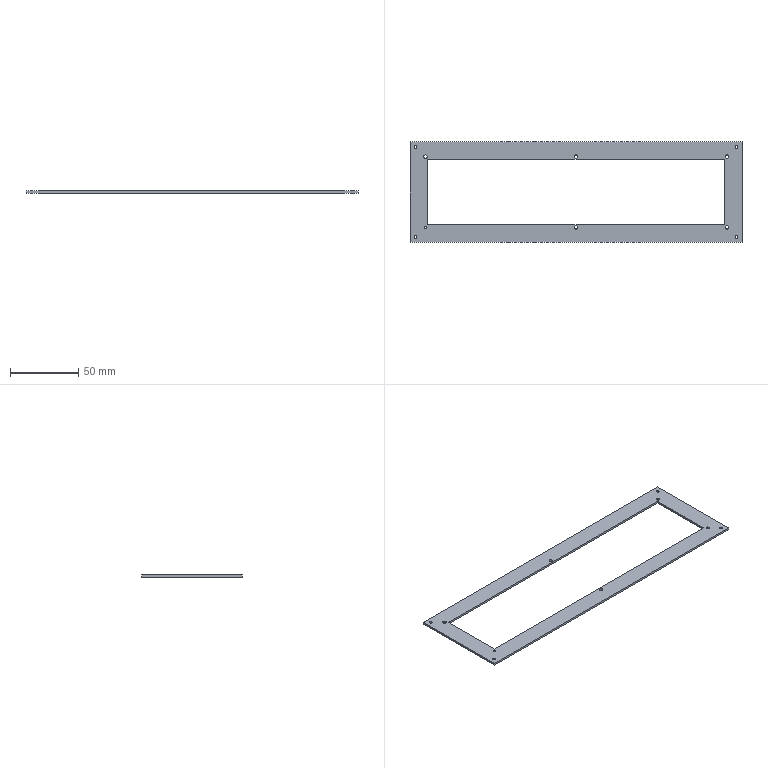Part | STEP file | FHD-021-001-R rack welded part R | 1 solid | 20 faces | box 244 x 74 x 1.5 mm | volume 11328 mm3 | plane 10 | cylinder 10 | commonest cylinder face diameters 2 x5 2.5 x5